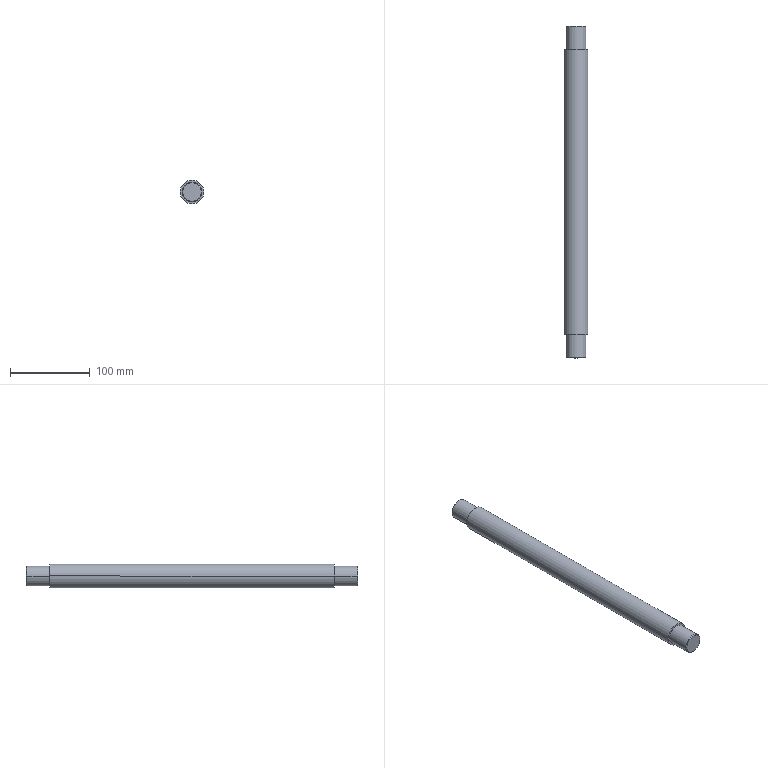Part | STEP file | ROLLER.SHAFT.IDLE.1.stp | 1 solid | 14 faces | box 30 x 416 x 30 mm | volume 281205 mm3 | spline 10 | plane 2 | cone 2